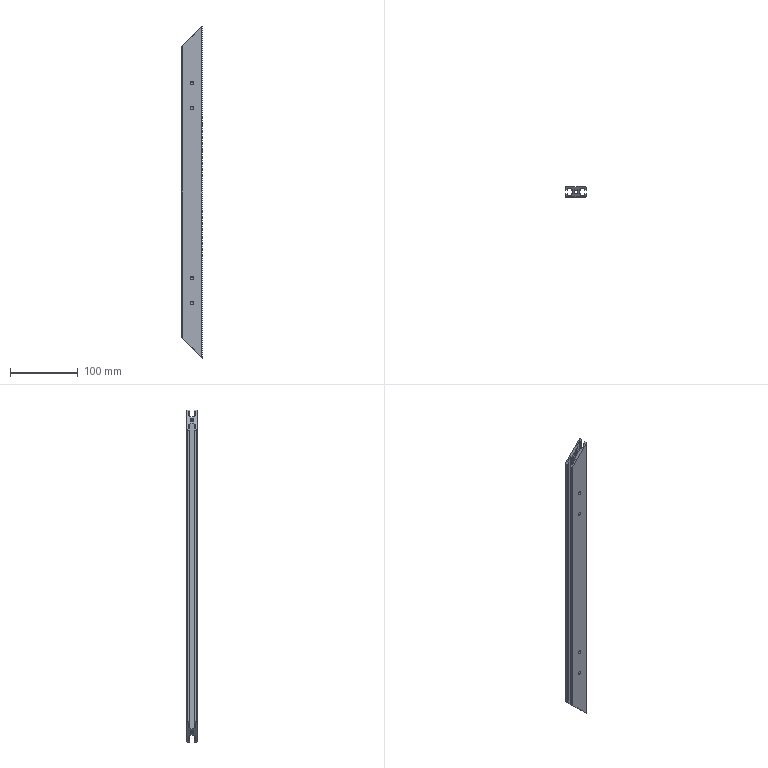Part | NX | features BREP 1 | 1 solid | 129 faces | box 30 x 15 x 491.9 mm | volume 110786 mm3 | cylinder 67 | plane 54 | cone 8 | commonest cylinder face diameters 5 x57 1 x6 2 x4